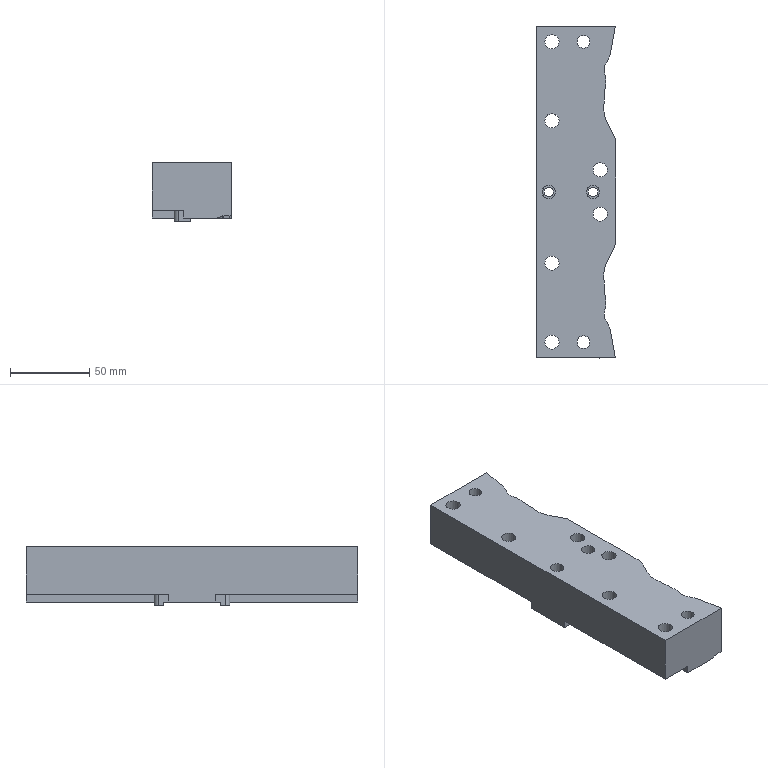Part | STEP file | PN_0035_id190_x_t | 1 solid | 104 faces | box 50.466 x 210 x 37 mm | volume 295873 mm3 | plane 44 | spline 36 | cylinder 24 | commonest cylinder face diameters 9 x6 14 x6 6 x4 8 x3 8.2 x2 8.5 x2